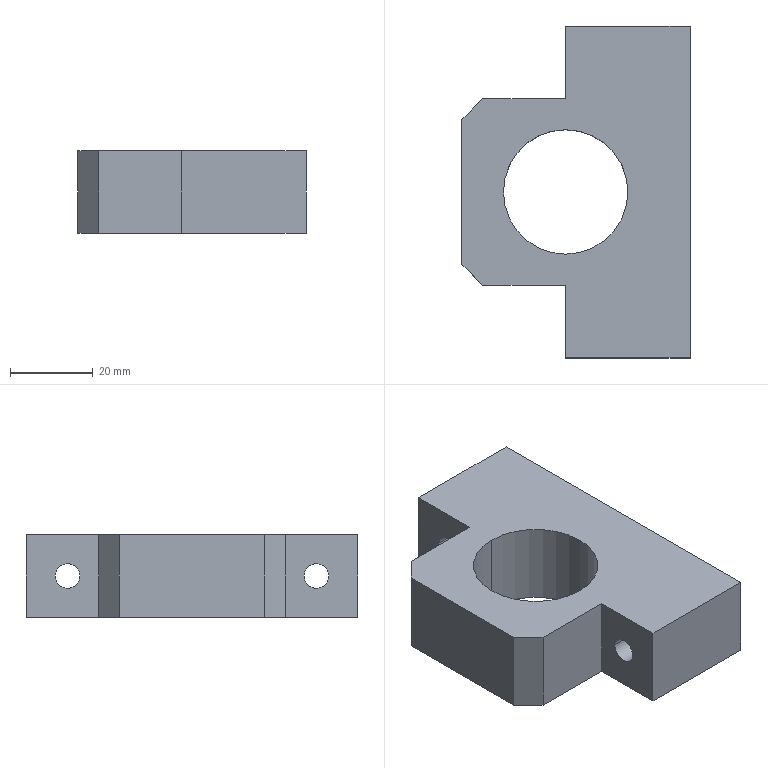Part | STEP file | Chamfer 1-13 | 1 solid | 18 faces | box 55 x 80 x 20 mm | volume 54166 mm3 | plane 12 | cylinder 6 | commonest cylinder face diameters 6 x4 30 x2
STEP:
#1=CARTESIAN_POINT('',(-1358.738,1767.264,3013.5));
#2=VERTEX_POINT('',#1);
#3=CARTESIAN_POINT('',(-1358.738,1761.264,3013.5));
#4=VERTEX_POINT('',#3);
#5=CARTESIAN_POINT('',(-1358.738,1764.264,3013.5));
#6=DIRECTION('',(-1.,0.,0.));
#7=DIRECTION('',(0.,-1.,0.));
#8=AXIS2_PLACEMENT_3D('',#5,#6,#7);
#9=CIRCLE('',#8,3.);
#10=EDGE_CURVE('',#2,#4,#9,.T.);
#11=ORIENTED_EDGE('',*,*,#10,.F.);
#12=CARTESIAN_POINT('',(-1388.738,1767.264,3013.5));
#13=VERTEX_POINT('',#12);
#14=CARTESIAN_POINT('',(-1311.738,1767.264,3013.5));
#15=DIRECTION('',(1.,0.,0.));
#16=VECTOR('',#15,1000.);
#17=LINE('',#14,#16);
#18=EDGE_CURVE('',#13,#2,#17,.T.);
#19=ORIENTED_EDGE('',*,*,#18,.F.);
#20=CARTESIAN_POINT('',(-1388.738,1761.264,3013.5));
#21=VERTEX_POINT('',#20);
#22=CARTESIAN_POINT('',(-1388.738,1764.264,3013.5));
#23=DIRECTION('',(-1.,0.,0.));
#24=DIRECTION('',(0.,-1.,0.));
#25=AXIS2_PLACEMENT_3D('',#22,#23,#24);
#26=CIRCLE('',#25,3.);
#27=EDGE_CURVE('',#13,#21,#26,.T.);
#28=ORIENTED_EDGE('',*,*,#27,.T.);
#29=CARTESIAN_POINT('',(-1311.738,1761.264,3013.5));
#30=DIRECTION('',(1.,0.,0.));
#31=VECTOR('',#30,1000.);
#32=LINE('',#29,#31);
#33=EDGE_CURVE('',#21,#4,#32,.T.);
#34=ORIENTED_EDGE('',*,*,#33,.T.);
#35=EDGE_LOOP('',(#11,#19,#28,#34));
#36=FACE_OUTER_BOUND('',#35,.T.);
#37=CARTESIAN_POINT('',(-1311.738,1764.264,3013.5));
#38=DIRECTION('',(-1.,0.,0.));
#39=DIRECTION('',(0.,1.,0.));
#40=AXIS2_PLACEMENT_3D('',#37,#38,#39);
#41=CYLINDRICAL_SURFACE('',#40,3.);
#42=ADVANCED_FACE('',(#36),#41,.F.);
#43=CARTESIAN_POINT('',(-1358.738,1707.264,3013.5));
#44=VERTEX_POINT('',#43);
#45=CARTESIAN_POINT('',(-1358.738,1701.264,3013.5));
#46=VERTEX_POINT('',#45);
#47=CARTESIAN_POINT('',(-1358.738,1704.264,3013.5));
#48=DIRECTION('',(-1.,0.,0.));
#49=DIRECTION('',(0.,-1.,0.));
#50=AXIS2_PLACEMENT_3D('',#47,#48,#49);
#51=CIRCLE('',#50,3.);
#52=EDGE_CURVE('',#44,#46,#51,.T.);
#53=ORIENTED_EDGE('',*,*,#52,.F.);
#54=CARTESIAN_POINT('',(-1388.738,1707.264,3013.5));
#55=VERTEX_POINT('',#54);
#56=CARTESIAN_POINT('',(-1311.738,1707.264,3013.5));
#57=DIRECTION('',(1.,0.,0.));
#58=VECTOR('',#57,1000.);
#59=LINE('',#56,#58);
#60=EDGE_CURVE('',#55,#44,#59,.T.);
#61=ORIENTED_EDGE('',*,*,#60,.F.);
#62=CARTESIAN_POINT('',(-1388.738,1701.264,3013.5));
#63=VERTEX_POINT('',#62);
#64=CARTESIAN_POINT('',(-1388.738,1704.264,3013.5));
#65=DIRECTION('',(-1.,0.,0.));
#66=DIRECTION('',(0.,-1.,0.));
#67=AXIS2_PLACEMENT_3D('',#64,#65,#66);
#68=CIRCLE('',#67,3.);
#69=EDGE_CURVE('',#55,#63,#68,.T.);
#70=ORIENTED_EDGE('',*,*,#69,.T.);
#71=CARTESIAN_POINT('',(-1311.738,1701.264,3013.5));
#72=DIRECTION('',(1.,0.,0.));
#73=VECTOR('',#72,1000.);
#74=LINE('',#71,#73);
#75=EDGE_CURVE('',#63,#46,#74,.T.);
#76=ORIENTED_EDGE('',*,*,#75,.T.);
#77=EDGE_LOOP('',(#53,#61,#70,#76));
#78=FACE_OUTER_BOUND('',#77,.T.);
#79=CARTESIAN_POINT('',(-1311.738,1704.264,3013.5));
#80=DIRECTION('',(-1.,0.,0.));
#81=DIRECTION('',(0.,1.,0.));
#82=AXIS2_PLACEMENT_3D('',#79,#80,#81);
#83=CYLINDRICAL_SURFACE('',#82,3.);
#84=ADVANCED_FACE('',(#78),#83,.F.);
#85=CARTESIAN_POINT('',(-1388.738,1719.264,3023.5));
#86=VERTEX_POINT('',#85);
#87=CARTESIAN_POINT('',(-1388.738,1749.264,3023.5));
#88=VERTEX_POINT('',#87);
#89=CARTESIAN_POINT('',(-1388.738,1734.264,3023.5));
#90=DIRECTION('',(0.,0.,1.));
#91=DIRECTION('',(0.,1.,0.));
#92=AXIS2_PLACEMENT_3D('',#89,#90,#91);
#93=CIRCLE('',#92,15.);
#94=EDGE_CURVE('',#86,#88,#93,.T.);
#95=ORIENTED_EDGE('',*,*,#94,.T.);
#96=CARTESIAN_POINT('',(-1388.738,1749.264,3003.5));
#97=VERTEX_POINT('',#96);
#98=CARTESIAN_POINT('',(-1388.738,1749.264,3023.5));
#99=DIRECTION('',(0.,0.,1.));
#100=VECTOR('',#99,1000.);
#101=LINE('',#98,#100);
#102=EDGE_CURVE('',#97,#88,#101,.T.);
#103=ORIENTED_EDGE('',*,*,#102,.F.);
#104=CARTESIAN_POINT('',(-1388.738,1719.264,3003.5));
#105=VERTEX_POINT('',#104);
#106=CARTESIAN_POINT('',(-1388.738,1734.264,3003.5));
#107=DIRECTION('',(0.,0.,1.));
#108=DIRECTION('',(0.,1.,0.));
#109=AXIS2_PLACEMENT_3D('',#106,#107,#108);
#110=CIRCLE('',#109,15.);
#111=EDGE_CURVE('',#105,#97,#110,.T.);
#112=ORIENTED_EDGE('',*,*,#111,.F.);
#113=CARTESIAN_POINT('',(-1388.738,1719.264,3023.5));
#114=DIRECTION('',(0.,0.,1.));
#115=VECTOR('',#114,1000.);
#116=LINE('',#113,#115);
#117=EDGE_CURVE('',#105,#86,#116,.T.);
#118=ORIENTED_EDGE('',*,*,#117,.T.);
#119=EDGE_LOOP('',(#95,#103,#112,#118));
#120=FACE_OUTER_BOUND('',#119,.T.);
#121=CARTESIAN_POINT('',(-1388.738,1734.264,3023.5));
#122=DIRECTION('',(0.,0.,-1.));
#123=DIRECTION('',(0.,1.,0.));
#124=AXIS2_PLACEMENT_3D('',#121,#122,#123);
#125=CYLINDRICAL_SURFACE('',#124,15.);
#126=ADVANCED_FACE('',(#120),#125,.F.);
#127=CARTESIAN_POINT('',(-1388.738,1756.764,3023.5));
#128=VERTEX_POINT('',#127);
#129=CARTESIAN_POINT('',(-1408.738,1756.764,3023.5));
#130=VERTEX_POINT('',#129);
#131=CARTESIAN_POINT('',(-1413.738,1756.764,3023.5));
#132=DIRECTION('',(-1.,0.,0.));
#133=VECTOR('',#132,1000.);
#134=LINE('',#131,#133);
#135=EDGE_CURVE('',#128,#130,#134,.T.);
#136=ORIENTED_EDGE('',*,*,#135,.T.);
#137=CARTESIAN_POINT('',(-1413.738,1751.764,3023.5));
#138=VERTEX_POINT('',#137);
#139=CARTESIAN_POINT('',(-1409.988,1755.514,3023.5));
#140=DIRECTION('',(-0.7071,-0.7071,0.));
#141=VECTOR('',#140,1000.);
#142=LINE('',#139,#141);
#143=EDGE_CURVE('',#130,#138,#142,.T.);
#144=ORIENTED_EDGE('',*,*,#143,.T.);
#145=CARTESIAN_POINT('',(-1413.738,1716.764,3023.5));
#146=VERTEX_POINT('',#145);
#147=CARTESIAN_POINT('',(-1413.738,1711.764,3023.5));
#148=DIRECTION('',(0.,-1.,0.));
#149=VECTOR('',#148,1000.);
#150=LINE('',#147,#149);
#151=EDGE_CURVE('',#138,#146,#150,.T.);
#152=ORIENTED_EDGE('',*,*,#151,.T.);
#153=CARTESIAN_POINT('',(-1408.738,1711.764,3023.5));
#154=VERTEX_POINT('',#153);
#155=CARTESIAN_POINT('',(-1409.988,1713.014,3023.5));
#156=DIRECTION('',(0.7071,-0.7071,0.));
#157=VECTOR('',#156,1000.);
#158=LINE('',#155,#157);
#159=EDGE_CURVE('',#146,#154,#158,.T.);
#160=ORIENTED_EDGE('',*,*,#159,.T.);
#161=CARTESIAN_POINT('',(-1388.738,1711.764,3023.5));
#162=VERTEX_POINT('',#161);
#163=CARTESIAN_POINT('',(-1388.738,1711.764,3023.5));
#164=DIRECTION('',(1.,0.,0.));
#165=VECTOR('',#164,1000.);
#166=LINE('',#163,#165);
#167=EDGE_CURVE('',#154,#162,#166,.T.);
#168=ORIENTED_EDGE('',*,*,#167,.T.);
#169=CARTESIAN_POINT('',(-1388.738,1694.264,3023.5));
#170=VERTEX_POINT('',#169);
#171=CARTESIAN_POINT('',(-1388.738,1694.264,3023.5));
#172=DIRECTION('',(0.,-1.,0.));
#173=VECTOR('',#172,1000.);
#174=LINE('',#171,#173);
#175=EDGE_CURVE('',#162,#170,#174,.T.);
#176=ORIENTED_EDGE('',*,*,#175,.T.);
#177=CARTESIAN_POINT('',(-1358.738,1694.264,3023.5));
#178=VERTEX_POINT('',#177);
#179=CARTESIAN_POINT('',(-1388.738,1694.264,3023.5));
#180=DIRECTION('',(1.,0.,0.));
#181=VECTOR('',#180,1000.);
#182=LINE('',#179,#181);
#183=EDGE_CURVE('',#170,#178,#182,.T.);
#184=ORIENTED_EDGE('',*,*,#183,.T.);
#185=CARTESIAN_POINT('',(-1358.738,1774.264,3023.5));
#186=VERTEX_POINT('',#185);
#187=CARTESIAN_POINT('',(-1358.738,1694.264,3023.5));
#188=DIRECTION('',(0.,1.,0.));
#189=VECTOR('',#188,1000.);
#190=LINE('',#187,#189);
#191=EDGE_CURVE('',#178,#186,#190,.T.);
#192=ORIENTED_EDGE('',*,*,#191,.T.);
#193=CARTESIAN_POINT('',(-1388.738,1774.264,3023.5));
#194=VERTEX_POINT('',#193);
#195=CARTESIAN_POINT('',(-1388.738,1774.264,3023.5));
#196=DIRECTION('',(-1.,0.,0.));
#197=VECTOR('',#196,1000.);
#198=LINE('',#195,#197);
#199=EDGE_CURVE('',#186,#194,#198,.T.);
#200=ORIENTED_EDGE('',*,*,#199,.T.);
#201=CARTESIAN_POINT('',(-1388.738,1756.764,3023.5));
#202=DIRECTION('',(0.,-1.,0.));
#203=VECTOR('',#202,1000.);
#204=LINE('',#201,#203);
#205=EDGE_CURVE('',#194,#128,#204,.T.);
#206=ORIENTED_EDGE('',*,*,#205,.T.);
#207=EDGE_LOOP('',(#136,#144,#152,#160,#168,#176,#184,#192,#200,#206));
#208=FACE_OUTER_BOUND('',#207,.T.);
#209=ORIENTED_EDGE('',*,*,#94,.F.);
#210=CARTESIAN_POINT('',(-1388.738,1734.264,3023.5));
#211=DIRECTION('',(0.,0.,1.));
#212=DIRECTION('',(0.,1.,0.));
#213=AXIS2_PLACEMENT_3D('',#210,#211,#212);
#214=CIRCLE('',#213,15.);
#215=EDGE_CURVE('',#88,#86,#214,.T.);
#216=ORIENTED_EDGE('',*,*,#215,.F.);
#217=EDGE_LOOP('',(#209,#216));
#218=FACE_BOUND('',#217,.T.);
#219=CARTESIAN_POINT('',(-1388.738,1734.264,3023.5));
#220=DIRECTION('',(0.,0.,1.));
#221=DIRECTION('',(0.,-1.,0.));
#222=AXIS2_PLACEMENT_3D('',#219,#220,#221);
#223=PLANE('',#222);
#224=ADVANCED_FACE('',(#208,#218),#223,.T.);
#225=CARTESIAN_POINT('',(-1413.738,1751.764,3003.5));
#226=VERTEX_POINT('',#225);
#227=CARTESIAN_POINT('',(-1413.738,1716.764,3003.5));
#228=VERTEX_POINT('',#227);
#229=CARTESIAN_POINT('',(-1413.738,1711.764,3003.5));
#230=DIRECTION('',(0.,-1.,0.));
#231=VECTOR('',#230,1000.);
#232=LINE('',#229,#231);
#233=EDGE_CURVE('',#226,#228,#232,.T.);
#234=ORIENTED_EDGE('',*,*,#233,.F.);
#235=CARTESIAN_POINT('',(-1408.738,1756.764,3003.5));
#236=VERTEX_POINT('',#235);
#237=CARTESIAN_POINT('',(-1413.738,1751.764,3003.5));
#238=DIRECTION('',(0.7071,0.7071,0.));
#239=VECTOR('',#238,1000.);
#240=LINE('',#237,#239);
#241=EDGE_CURVE('',#226,#236,#240,.T.);
#242=ORIENTED_EDGE('',*,*,#241,.T.);
#243=CARTESIAN_POINT('',(-1388.738,1756.764,3003.5));
#244=VERTEX_POINT('',#243);
#245=CARTESIAN_POINT('',(-1413.738,1756.764,3003.5));
#246=DIRECTION('',(-1.,0.,0.));
#247=VECTOR('',#246,1000.);
#248=LINE('',#245,#247);
#249=EDGE_CURVE('',#244,#236,#248,.T.);
#250=ORIENTED_EDGE('',*,*,#249,.F.);
#251=CARTESIAN_POINT('',(-1388.738,1774.264,3003.5));
#252=VERTEX_POINT('',#251);
#253=CARTESIAN_POINT('',(-1388.738,1756.764,3003.5));
#254=DIRECTION('',(0.,-1.,0.));
#255=VECTOR('',#254,1000.);
#256=LINE('',#253,#255);
#257=EDGE_CURVE('',#252,#244,#256,.T.);
#258=ORIENTED_EDGE('',*,*,#257,.F.);
#259=CARTESIAN_POINT('',(-1358.738,1774.264,3003.5));
#260=VERTEX_POINT('',#259);
#261=CARTESIAN_POINT('',(-1388.738,1774.264,3003.5));
#262=DIRECTION('',(-1.,0.,0.));
#263=VECTOR('',#262,1000.);
#264=LINE('',#261,#263);
#265=EDGE_CURVE('',#260,#252,#264,.T.);
#266=ORIENTED_EDGE('',*,*,#265,.F.);
#267=CARTESIAN_POINT('',(-1358.738,1694.264,3003.5));
#268=VERTEX_POINT('',#267);
#269=CARTESIAN_POINT('',(-1358.738,1694.264,3003.5));
#270=DIRECTION('',(0.,1.,0.));
#271=VECTOR('',#270,1000.);
#272=LINE('',#269,#271);
#273=EDGE_CURVE('',#268,#260,#272,.T.);
#274=ORIENTED_EDGE('',*,*,#273,.F.);
#275=CARTESIAN_POINT('',(-1388.738,1694.264,3003.5));
#276=VERTEX_POINT('',#275);
#277=CARTESIAN_POINT('',(-1388.738,1694.264,3003.5));
#278=DIRECTION('',(1.,0.,0.));
#279=VECTOR('',#278,1000.);
#280=LINE('',#277,#279);
#281=EDGE_CURVE('',#276,#268,#280,.T.);
#282=ORIENTED_EDGE('',*,*,#281,.F.);
#283=CARTESIAN_POINT('',(-1388.738,1711.764,3003.5));
#284=VERTEX_POINT('',#283);
#285=CARTESIAN_POINT('',(-1388.738,1694.264,3003.5));
#286=DIRECTION('',(0.,-1.,0.));
#287=VECTOR('',#286,1000.);
#288=LINE('',#285,#287);
#289=EDGE_CURVE('',#284,#276,#288,.T.);
#290=ORIENTED_EDGE('',*,*,#289,.F.);
#291=CARTESIAN_POINT('',(-1408.738,1711.764,3003.5));
#292=VERTEX_POINT('',#291);
#293=CARTESIAN_POINT('',(-1388.738,1711.764,3003.5));
#294=DIRECTION('',(1.,0.,0.));
#295=VECTOR('',#294,1000.);
#296=LINE('',#293,#295);
#297=EDGE_CURVE('',#292,#284,#296,.T.);
#298=ORIENTED_EDGE('',*,*,#297,.F.);
#299=CARTESIAN_POINT('',(-1408.738,1711.764,3003.5));
#300=DIRECTION('',(-0.7071,0.7071,0.));
#301=VECTOR('',#300,1000.);
#302=LINE('',#299,#301);
#303=EDGE_CURVE('',#292,#228,#302,.T.);
#304=ORIENTED_EDGE('',*,*,#303,.T.);
#305=EDGE_LOOP('',(#234,#242,#250,#258,#266,#274,#282,#290,#298,#304));
#306=FACE_OUTER_BOUND('',#305,.T.);
#307=ORIENTED_EDGE('',*,*,#111,.T.);
#308=CARTESIAN_POINT('',(-1388.738,1734.264,3003.5));
#309=DIRECTION('',(0.,0.,1.));
#310=DIRECTION('',(0.,1.,0.));
#311=AXIS2_PLACEMENT_3D('',#308,#309,#310);
#312=CIRCLE('',#311,15.);
#313=EDGE_CURVE('',#97,#105,#312,.T.);
#314=ORIENTED_EDGE('',*,*,#313,.T.);
#315=EDGE_LOOP('',(#307,#314));
#316=FACE_BOUND('',#315,.T.);
#317=CARTESIAN_POINT('',(-1388.738,1734.264,3003.5));
#318=DIRECTION('',(0.,0.,1.));
#319=DIRECTION('',(0.,-1.,0.));
#320=AXIS2_PLACEMENT_3D('',#317,#318,#319);
#321=PLANE('',#320);
#322=ADVANCED_FACE('',(#306,#316),#321,.F.);
#323=ORIENTED_EDGE('',*,*,#281,.T.);
#324=CARTESIAN_POINT('',(-1358.738,1694.264,3023.5));
#325=DIRECTION('',(0.,0.,-1.));
#326=VECTOR('',#325,1000.);
#327=LINE('',#324,#326);
#328=EDGE_CURVE('',#178,#268,#327,.T.);
#329=ORIENTED_EDGE('',*,*,#328,.F.);
#330=ORIENTED_EDGE('',*,*,#183,.F.);
#331=CARTESIAN_POINT('',(-1388.738,1694.264,3023.5));
#332=DIRECTION('',(0.,0.,-1.));
#333=VECTOR('',#332,1000.);
#334=LINE('',#331,#333);
#335=EDGE_CURVE('',#170,#276,#334,.T.);
#336=ORIENTED_EDGE('',*,*,#335,.T.);
#337=EDGE_LOOP('',(#323,#329,#330,#336));
#338=FACE_OUTER_BOUND('',#337,.T.);
#339=CARTESIAN_POINT('',(-1388.738,1694.264,3023.5));
#340=DIRECTION('',(0.,1.,0.));
#341=DIRECTION('',(1.,0.,0.));
#342=AXIS2_PLACEMENT_3D('',#339,#340,#341);
#343=PLANE('',#342);
#344=ADVANCED_FACE('',(#338),#343,.F.);
#345=CARTESIAN_POINT('',(-1358.738,1764.264,3013.5));
#346=DIRECTION('',(-1.,0.,0.));
#347=DIRECTION('',(0.,-1.,0.));
#348=AXIS2_PLACEMENT_3D('',#345,#346,#347);
#349=CIRCLE('',#348,3.);
#350=EDGE_CURVE('',#4,#2,#349,.T.);
#351=ORIENTED_EDGE('',*,*,#350,.T.);
#352=ORIENTED_EDGE('',*,*,#10,.T.);
#353=EDGE_LOOP('',(#351,#352));
#354=FACE_BOUND('',#353,.T.);
#355=CARTESIAN_POINT('',(-1358.738,1704.264,3013.5));
#356=DIRECTION('',(-1.,0.,0.));
#357=DIRECTION('',(0.,-1.,0.));
#358=AXIS2_PLACEMENT_3D('',#355,#356,#357);
#359=CIRCLE('',#358,3.);
#360=EDGE_CURVE('',#46,#44,#359,.T.);
#361=ORIENTED_EDGE('',*,*,#360,.T.);
#362=ORIENTED_EDGE('',*,*,#52,.T.);
#363=EDGE_LOOP('',(#361,#362));
#364=FACE_BOUND('',#363,.T.);
#365=ORIENTED_EDGE('',*,*,#273,.T.);
#366=CARTESIAN_POINT('',(-1358.738,1774.264,3023.5));
#367=DIRECTION('',(0.,0.,-1.));
#368=VECTOR('',#367,1000.);
#369=LINE('',#366,#368);
#370=EDGE_CURVE('',#186,#260,#369,.T.);
#371=ORIENTED_EDGE('',*,*,#370,.F.);
#372=ORIENTED_EDGE('',*,*,#191,.F.);
#373=ORIENTED_EDGE('',*,*,#328,.T.);
#374=EDGE_LOOP('',(#365,#371,#372,#373));
#375=FACE_OUTER_BOUND('',#374,.T.);
#376=CARTESIAN_POINT('',(-1358.738,1694.264,3023.5));
#377=DIRECTION('',(-1.,0.,0.));
#378=DIRECTION('',(0.,1.,0.));
#379=AXIS2_PLACEMENT_3D('',#376,#377,#378);
#380=PLANE('',#379);
#381=ADVANCED_FACE('',(#354,#364,#375),#380,.F.);
#382=ORIENTED_EDGE('',*,*,#265,.T.);
#383=CARTESIAN_POINT('',(-1388.738,1774.264,3023.5));
#384=DIRECTION('',(0.,0.,-1.));
#385=VECTOR('',#384,1000.);
#386=LINE('',#383,#385);
#387=EDGE_CURVE('',#194,#252,#386,.T.);
#388=ORIENTED_EDGE('',*,*,#387,.F.);
#389=ORIENTED_EDGE('',*,*,#199,.F.);
#390=ORIENTED_EDGE('',*,*,#370,.T.);
#391=EDGE_LOOP('',(#382,#388,#389,#390));
#392=FACE_OUTER_BOUND('',#391,.T.);
#393=CARTESIAN_POINT('',(-1388.738,1774.264,3023.5));
#394=DIRECTION('',(0.,-1.,0.));
#395=DIRECTION('',(-1.,0.,0.));
#396=AXIS2_PLACEMENT_3D('',#393,#394,#395);
#397=PLANE('',#396);
#398=ADVANCED_FACE('',(#392),#397,.F.);
#399=CARTESIAN_POINT('',(-1388.738,1764.264,3013.5));
#400=DIRECTION('',(-1.,0.,0.));
#401=DIRECTION('',(0.,-1.,0.));
#402=AXIS2_PLACEMENT_3D('',#399,#400,#401);
#403=CIRCLE('',#402,3.);
#404=EDGE_CURVE('',#21,#13,#403,.T.);
#405=ORIENTED_EDGE('',*,*,#404,.F.);
#406=ORIENTED_EDGE('',*,*,#27,.F.);
#407=EDGE_LOOP('',(#405,#406));
#408=FACE_BOUND('',#407,.T.);
#409=ORIENTED_EDGE('',*,*,#257,.T.);
#410=CARTESIAN_POINT('',(-1388.738,1756.764,3023.5));
#411=DIRECTION('',(0.,0.,-1.));
#412=VECTOR('',#411,1000.);
#413=LINE('',#410,#412);
#414=EDGE_CURVE('',#128,#244,#413,.T.);
#415=ORIENTED_EDGE('',*,*,#414,.F.);
#416=ORIENTED_EDGE('',*,*,#205,.F.);
#417=ORIENTED_EDGE('',*,*,#387,.T.);
#418=EDGE_LOOP('',(#409,#415,#416,#417));
#419=FACE_OUTER_BOUND('',#418,.T.);
#420=CARTESIAN_POINT('',(-1388.738,1756.764,3023.5));
#421=DIRECTION('',(1.,0.,0.));
#422=DIRECTION('',(0.,0.,1.));
#423=AXIS2_PLACEMENT_3D('',#420,#421,#422);
#424=PLANE('',#423);
#425=ADVANCED_FACE('',(#408,#419),#424,.F.);
#426=ORIENTED_EDGE('',*,*,#249,.T.);
#427=CARTESIAN_POINT('',(-1408.738,1756.764,3023.5));
#428=DIRECTION('',(0.,0.,1.));
#429=VECTOR('',#428,1000.);
#430=LINE('',#427,#429);
#431=EDGE_CURVE('',#236,#130,#430,.T.);
#432=ORIENTED_EDGE('',*,*,#431,.T.);
#433=ORIENTED_EDGE('',*,*,#135,.F.);
#434=ORIENTED_EDGE('',*,*,#414,.T.);
#435=EDGE_LOOP('',(#426,#432,#433,#434));
#436=FACE_OUTER_BOUND('',#435,.T.);
#437=CARTESIAN_POINT('',(-1413.738,1756.764,3023.5));
#438=DIRECTION('',(0.,-1.,0.));
#439=DIRECTION('',(-1.,0.,0.));
#440=AXIS2_PLACEMENT_3D('',#437,#438,#439);
#441=PLANE('',#440);
#442=ADVANCED_FACE('',(#436),#441,.F.);
#443=ORIENTED_EDGE('',*,*,#151,.F.);
#444=CARTESIAN_POINT('',(-1413.738,1751.764,3023.5));
#445=DIRECTION('',(0.,0.,-1.));
#446=VECTOR('',#445,1000.);
#447=LINE('',#444,#446);
#448=EDGE_CURVE('',#138,#226,#447,.T.);
#449=ORIENTED_EDGE('',*,*,#448,.T.);
#450=ORIENTED_EDGE('',*,*,#233,.T.);
#451=CARTESIAN_POINT('',(-1413.738,1716.764,3023.5));
#452=DIRECTION('',(0.,0.,1.));
#453=VECTOR('',#452,1000.);
#454=LINE('',#451,#453);
#455=EDGE_CURVE('',#228,#146,#454,.T.);
#456=ORIENTED_EDGE('',*,*,#455,.T.);
#457=EDGE_LOOP('',(#443,#449,#450,#456));
#458=FACE_OUTER_BOUND('',#457,.T.);
#459=CARTESIAN_POINT('',(-1413.738,1711.764,3023.5));
#460=DIRECTION('',(1.,0.,0.));
#461=DIRECTION('',(0.,0.,1.));
#462=AXIS2_PLACEMENT_3D('',#459,#460,#461);
#463=PLANE('',#462);
#464=ADVANCED_FACE('',(#458),#463,.F.);
#465=ORIENTED_EDGE('',*,*,#167,.F.);
#466=CARTESIAN_POINT('',(-1408.738,1711.764,3023.5));
#467=DIRECTION('',(0.,0.,-1.));
#468=VECTOR('',#467,1000.);
#469=LINE('',#466,#468);
#470=EDGE_CURVE('',#154,#292,#469,.T.);
#471=ORIENTED_EDGE('',*,*,#470,.T.);
#472=ORIENTED_EDGE('',*,*,#297,.T.);
#473=CARTESIAN_POINT('',(-1388.738,1711.764,3023.5));
#474=DIRECTION('',(0.,0.,-1.));
#475=VECTOR('',#474,1000.);
#476=LINE('',#473,#475);
#477=EDGE_CURVE('',#162,#284,#476,.T.);
#478=ORIENTED_EDGE('',*,*,#477,.F.);
#479=EDGE_LOOP('',(#465,#471,#472,#478));
#480=FACE_OUTER_BOUND('',#479,.T.);
#481=CARTESIAN_POINT('',(-1388.738,1711.764,3023.5));
#482=DIRECTION('',(0.,1.,0.));
#483=DIRECTION('',(0.,0.,1.));
#484=AXIS2_PLACEMENT_3D('',#481,#482,#483);
#485=PLANE('',#484);
#486=ADVANCED_FACE('',(#480),#485,.F.);
#487=CARTESIAN_POINT('',(-1388.738,1704.264,3013.5));
#488=DIRECTION('',(-1.,0.,0.));
#489=DIRECTION('',(0.,-1.,0.));
#490=AXIS2_PLACEMENT_3D('',#487,#488,#489);
#491=CIRCLE('',#490,3.);
#492=EDGE_CURVE('',#63,#55,#491,.T.);
#493=ORIENTED_EDGE('',*,*,#492,.F.);
#494=ORIENTED_EDGE('',*,*,#69,.F.);
#495=EDGE_LOOP('',(#493,#494));
#496=FACE_BOUND('',#495,.T.);
#497=ORIENTED_EDGE('',*,*,#289,.T.);
#498=ORIENTED_EDGE('',*,*,#335,.F.);
#499=ORIENTED_EDGE('',*,*,#175,.F.);
#500=ORIENTED_EDGE('',*,*,#477,.T.);
#501=EDGE_LOOP('',(#497,#498,#499,#500));
#502=FACE_OUTER_BOUND('',#501,.T.);
#503=CARTESIAN_POINT('',(-1388.738,1694.264,3023.5));
#504=DIRECTION('',(1.,0.,0.));
#505=DIRECTION('',(0.,0.,1.));
#506=AXIS2_PLACEMENT_3D('',#503,#504,#505);
#507=PLANE('',#506);
#508=ADVANCED_FACE('',(#496,#502),#507,.F.);
#509=ORIENTED_EDGE('',*,*,#102,.T.);
#510=ORIENTED_EDGE('',*,*,#215,.T.);
#511=ORIENTED_EDGE('',*,*,#117,.F.);
#512=ORIENTED_EDGE('',*,*,#313,.F.);
#513=EDGE_LOOP('',(#509,#510,#511,#512));
#514=FACE_OUTER_BOUND('',#513,.T.);
#515=CARTESIAN_POINT('',(-1388.738,1734.264,3023.5));
#516=DIRECTION('',(0.,0.,-1.));
#517=DIRECTION('',(0.,1.,0.));
#518=AXIS2_PLACEMENT_3D('',#515,#516,#517);
#519=CYLINDRICAL_SURFACE('',#518,15.);
#520=ADVANCED_FACE('',(#514),#519,.F.);
#521=ORIENTED_EDGE('',*,*,#60,.T.);
#522=ORIENTED_EDGE('',*,*,#360,.F.);
#523=ORIENTED_EDGE('',*,*,#75,.F.);
#524=ORIENTED_EDGE('',*,*,#492,.T.);
#525=EDGE_LOOP('',(#521,#522,#523,#524));
#526=FACE_OUTER_BOUND('',#525,.T.);
#527=CARTESIAN_POINT('',(-1311.738,1704.264,3013.5));
#528=DIRECTION('',(-1.,0.,0.));
#529=DIRECTION('',(0.,1.,0.));
#530=AXIS2_PLACEMENT_3D('',#527,#528,#529);
#531=CYLINDRICAL_SURFACE('',#530,3.);
#532=ADVANCED_FACE('',(#526),#531,.F.);
#533=ORIENTED_EDGE('',*,*,#18,.T.);
#534=ORIENTED_EDGE('',*,*,#350,.F.);
#535=ORIENTED_EDGE('',*,*,#33,.F.);
#536=ORIENTED_EDGE('',*,*,#404,.T.);
#537=EDGE_LOOP('',(#533,#534,#535,#536));
#538=FACE_OUTER_BOUND('',#537,.T.);
#539=CARTESIAN_POINT('',(-1311.738,1764.264,3013.5));
#540=DIRECTION('',(-1.,0.,0.));
#541=DIRECTION('',(0.,1.,0.));
#542=AXIS2_PLACEMENT_3D('',#539,#540,#541);
#543=CYLINDRICAL_SURFACE('',#542,3.);
#544=ADVANCED_FACE('',(#538),#543,.F.);
#545=ORIENTED_EDGE('',*,*,#143,.F.);
#546=ORIENTED_EDGE('',*,*,#431,.F.);
#547=ORIENTED_EDGE('',*,*,#241,.F.);
#548=ORIENTED_EDGE('',*,*,#448,.F.);
#549=EDGE_LOOP('',(#545,#546,#547,#548));
#550=FACE_OUTER_BOUND('',#549,.T.);
#551=CARTESIAN_POINT('',(-1413.738,1751.764,3023.5));
#552=DIRECTION('',(0.7071,-0.7071,0.));
#553=DIRECTION('',(0.,0.,1.));
#554=AXIS2_PLACEMENT_3D('',#551,#552,#553);
#555=PLANE('',#554);
#556=ADVANCED_FACE('',(#550),#555,.F.);
#557=ORIENTED_EDGE('',*,*,#159,.F.);
#558=ORIENTED_EDGE('',*,*,#455,.F.);
#559=ORIENTED_EDGE('',*,*,#303,.F.);
#560=ORIENTED_EDGE('',*,*,#470,.F.);
#561=EDGE_LOOP('',(#557,#558,#559,#560));
#562=FACE_OUTER_BOUND('',#561,.T.);
#563=CARTESIAN_POINT('',(-1408.738,1711.764,3023.5));
#564=DIRECTION('',(0.7071,0.7071,0.));
#565=DIRECTION('',(0.,0.,1.));
#566=AXIS2_PLACEMENT_3D('',#563,#564,#565);
#567=PLANE('',#566);
#568=ADVANCED_FACE('',(#562),#567,.F.);
#569=CLOSED_SHELL('',(#42,#84,#126,#224,#322,#344,#381,#398,#425,#442,#464,#486,#508,#520,#532,#544,#556,#568));
#570=MANIFOLD_SOLID_BREP('',#569);
#571=CARTESIAN_POINT('',(0.,0.,0.));
#572=DIRECTION('',(0.,0.,1.));
#573=DIRECTION('',(1.,0.,0.));
#574=AXIS2_PLACEMENT_3D('',#571,#572,#573);
#575=(LENGTH_UNIT()NAMED_UNIT(*)SI_UNIT(.MILLI.,.METRE.));
#576=UNCERTAINTY_MEASURE_WITH_UNIT(LENGTH_MEASURE(0.00001),#575,'','');
#577=(NAMED_UNIT(*)PLANE_ANGLE_UNIT()SI_UNIT($,.RADIAN.));
#578=(NAMED_UNIT(*)SI_UNIT($,.STERADIAN.)SOLID_ANGLE_UNIT());
#579=(GEOMETRIC_REPRESENTATION_CONTEXT(3)GLOBAL_UNCERTAINTY_ASSIGNED_CONTEXT((#576))GLOBAL_UNIT_ASSIGNED_CONTEXT((#575,#577,#578))REPRESENTATION_CONTEXT('',''));
#580=ADVANCED_BREP_SHAPE_REPRESENTATION('',(#570,#574),#579);